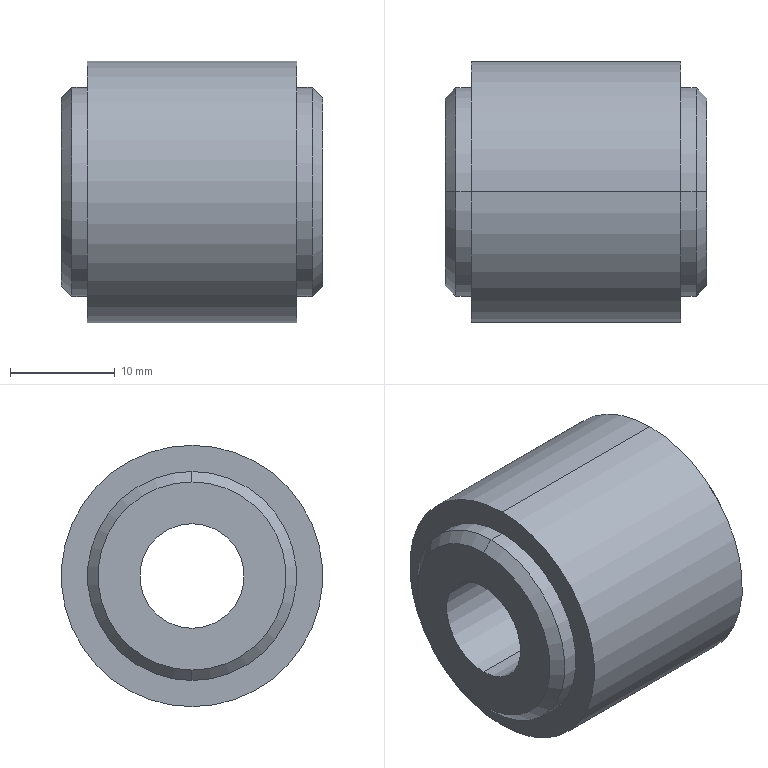Part | SolidWorks | features Chamfer 1, Extrusion 1, ICE 1 | 1 solid | 16 faces | box 25 x 25 x 25 mm | volume 9364 mm3 | cylinder 8 | cone 4 | plane 4 | commonest cylinder face diameters 20 x4 10 x2 25 x2
STEP:
#1=CARTESIAN_POINT('',(12.5,0.,-9.));
#2=VERTEX_POINT('',#1);
#3=CARTESIAN_POINT('',(12.5,0.,9.));
#4=VERTEX_POINT('',#3);
#5=CARTESIAN_POINT('',(12.5,0.,0.));
#6=DIRECTION('',(1.,0.,0.));
#7=DIRECTION('',(0.,0.,-1.));
#8=AXIS2_PLACEMENT_3D('',#5,#6,#7);
#9=CIRCLE('',#8,9.);
#10=EDGE_CURVE('',#2,#4,#9,.T.);
#11=ORIENTED_EDGE('',*,*,#10,.F.);
#12=CARTESIAN_POINT('',(11.5,0.,-10.));
#13=VERTEX_POINT('',#12);
#14=CARTESIAN_POINT('',(12.5,0.,-9.));
#15=DIRECTION('',(-0.7071,0.,-0.7071));
#16=VECTOR('',#15,1000.);
#17=LINE('',#14,#16);
#18=EDGE_CURVE('',#2,#13,#17,.T.);
#19=ORIENTED_EDGE('',*,*,#18,.T.);
#20=CARTESIAN_POINT('',(11.5,0.,10.));
#21=VERTEX_POINT('',#20);
#22=CARTESIAN_POINT('',(11.5,0.,0.));
#23=DIRECTION('',(-1.,0.,0.));
#24=DIRECTION('',(0.,0.,-1.));
#25=AXIS2_PLACEMENT_3D('',#22,#23,#24);
#26=CIRCLE('',#25,10.);
#27=EDGE_CURVE('',#21,#13,#26,.T.);
#28=ORIENTED_EDGE('',*,*,#27,.F.);
#29=CARTESIAN_POINT('',(12.5,0.,9.));
#30=DIRECTION('',(-0.7071,0.,0.7071));
#31=VECTOR('',#30,1000.);
#32=LINE('',#29,#31);
#33=EDGE_CURVE('',#4,#21,#32,.T.);
#34=ORIENTED_EDGE('',*,*,#33,.F.);
#35=EDGE_LOOP('',(#11,#19,#28,#34));
#36=FACE_OUTER_BOUND('',#35,.T.);
#37=CARTESIAN_POINT('',(12.5,0.,0.));
#38=DIRECTION('',(-1.,0.,0.));
#39=DIRECTION('',(0.,0.,1.));
#40=AXIS2_PLACEMENT_3D('',#37,#38,#39);
#41=CONICAL_SURFACE('',#40,9.,0.7854);
#42=ADVANCED_FACE('',(#36),#41,.T.);
#43=CARTESIAN_POINT('',(-12.5,0.,9.));
#44=VERTEX_POINT('',#43);
#45=CARTESIAN_POINT('',(-12.5,0.,-9.));
#46=VERTEX_POINT('',#45);
#47=CARTESIAN_POINT('',(-12.5,0.,0.));
#48=DIRECTION('',(-1.,0.,0.));
#49=DIRECTION('',(0.,0.,-1.));
#50=AXIS2_PLACEMENT_3D('',#47,#48,#49);
#51=CIRCLE('',#50,9.);
#52=EDGE_CURVE('',#44,#46,#51,.T.);
#53=ORIENTED_EDGE('',*,*,#52,.F.);
#54=CARTESIAN_POINT('',(-11.5,0.,10.));
#55=VERTEX_POINT('',#54);
#56=CARTESIAN_POINT('',(-11.5,0.,10.));
#57=DIRECTION('',(0.7071,0.,0.7071));
#58=VECTOR('',#57,1000.);
#59=LINE('',#56,#58);
#60=EDGE_CURVE('',#44,#55,#59,.T.);
#61=ORIENTED_EDGE('',*,*,#60,.T.);
#62=CARTESIAN_POINT('',(-11.5,0.,-10.));
#63=VERTEX_POINT('',#62);
#64=CARTESIAN_POINT('',(-11.5,0.,0.));
#65=DIRECTION('',(1.,0.,0.));
#66=DIRECTION('',(0.,0.,-1.));
#67=AXIS2_PLACEMENT_3D('',#64,#65,#66);
#68=CIRCLE('',#67,10.);
#69=EDGE_CURVE('',#63,#55,#68,.T.);
#70=ORIENTED_EDGE('',*,*,#69,.F.);
#71=CARTESIAN_POINT('',(-11.5,0.,-10.));
#72=DIRECTION('',(0.7071,0.,-0.7071));
#73=VECTOR('',#72,1000.);
#74=LINE('',#71,#73);
#75=EDGE_CURVE('',#46,#63,#74,.T.);
#76=ORIENTED_EDGE('',*,*,#75,.F.);
#77=EDGE_LOOP('',(#53,#61,#70,#76));
#78=FACE_OUTER_BOUND('',#77,.T.);
#79=CARTESIAN_POINT('',(-11.5,0.,0.));
#80=DIRECTION('',(1.,0.,0.));
#81=DIRECTION('',(0.,0.,-1.));
#82=AXIS2_PLACEMENT_3D('',#79,#80,#81);
#83=CONICAL_SURFACE('',#82,10.,0.7854);
#84=ADVANCED_FACE('',(#78),#83,.T.);
#85=CARTESIAN_POINT('',(10.,0.,-12.5));
#86=VERTEX_POINT('',#85);
#87=CARTESIAN_POINT('',(10.,0.,12.5));
#88=VERTEX_POINT('',#87);
#89=CARTESIAN_POINT('',(10.,0.,0.));
#90=DIRECTION('',(1.,0.,0.));
#91=DIRECTION('',(0.,0.,-1.));
#92=AXIS2_PLACEMENT_3D('',#89,#90,#91);
#93=CIRCLE('',#92,12.5);
#94=EDGE_CURVE('',#86,#88,#93,.T.);
#95=ORIENTED_EDGE('',*,*,#94,.F.);
#96=CARTESIAN_POINT('',(-10.,0.,-12.5));
#97=VERTEX_POINT('',#96);
#98=CARTESIAN_POINT('',(10.,0.,-12.5));
#99=DIRECTION('',(-1.,0.,0.));
#100=VECTOR('',#99,1000.);
#101=LINE('',#98,#100);
#102=EDGE_CURVE('',#86,#97,#101,.T.);
#103=ORIENTED_EDGE('',*,*,#102,.T.);
#104=CARTESIAN_POINT('',(-10.,0.,12.5));
#105=VERTEX_POINT('',#104);
#106=CARTESIAN_POINT('',(-10.,0.,0.));
#107=DIRECTION('',(1.,0.,0.));
#108=DIRECTION('',(0.,0.,-1.));
#109=AXIS2_PLACEMENT_3D('',#106,#107,#108);
#110=CIRCLE('',#109,12.5);
#111=EDGE_CURVE('',#97,#105,#110,.T.);
#112=ORIENTED_EDGE('',*,*,#111,.T.);
#113=CARTESIAN_POINT('',(10.,0.,12.5));
#114=DIRECTION('',(-1.,0.,0.));
#115=VECTOR('',#114,1000.);
#116=LINE('',#113,#115);
#117=EDGE_CURVE('',#88,#105,#116,.T.);
#118=ORIENTED_EDGE('',*,*,#117,.F.);
#119=EDGE_LOOP('',(#95,#103,#112,#118));
#120=FACE_OUTER_BOUND('',#119,.T.);
#121=CARTESIAN_POINT('',(10.,0.,0.));
#122=DIRECTION('',(-1.,0.,0.));
#123=DIRECTION('',(0.,0.,1.));
#124=AXIS2_PLACEMENT_3D('',#121,#122,#123);
#125=CYLINDRICAL_SURFACE('',#124,12.5);
#126=ADVANCED_FACE('',(#120),#125,.T.);
#127=CARTESIAN_POINT('',(12.5,0.,5.));
#128=VERTEX_POINT('',#127);
#129=CARTESIAN_POINT('',(12.5,0.,-5.));
#130=VERTEX_POINT('',#129);
#131=CARTESIAN_POINT('',(12.5,0.,0.));
#132=DIRECTION('',(1.,0.,0.));
#133=DIRECTION('',(0.,0.,-1.));
#134=AXIS2_PLACEMENT_3D('',#131,#132,#133);
#135=CIRCLE('',#134,5.);
#136=EDGE_CURVE('',#128,#130,#135,.T.);
#137=ORIENTED_EDGE('',*,*,#136,.T.);
#138=CARTESIAN_POINT('',(-12.5,0.,-5.));
#139=VERTEX_POINT('',#138);
#140=CARTESIAN_POINT('',(12.5,0.,-5.));
#141=DIRECTION('',(-1.,0.,0.));
#142=VECTOR('',#141,1000.);
#143=LINE('',#140,#142);
#144=EDGE_CURVE('',#130,#139,#143,.T.);
#145=ORIENTED_EDGE('',*,*,#144,.T.);
#146=CARTESIAN_POINT('',(-12.5,0.,5.));
#147=VERTEX_POINT('',#146);
#148=CARTESIAN_POINT('',(-12.5,0.,0.));
#149=DIRECTION('',(1.,0.,0.));
#150=DIRECTION('',(0.,0.,-1.));
#151=AXIS2_PLACEMENT_3D('',#148,#149,#150);
#152=CIRCLE('',#151,5.);
#153=EDGE_CURVE('',#147,#139,#152,.T.);
#154=ORIENTED_EDGE('',*,*,#153,.F.);
#155=CARTESIAN_POINT('',(12.5,0.,5.));
#156=DIRECTION('',(-1.,0.,0.));
#157=VECTOR('',#156,1000.);
#158=LINE('',#155,#157);
#159=EDGE_CURVE('',#128,#147,#158,.T.);
#160=ORIENTED_EDGE('',*,*,#159,.F.);
#161=EDGE_LOOP('',(#137,#145,#154,#160));
#162=FACE_OUTER_BOUND('',#161,.T.);
#163=CARTESIAN_POINT('',(12.5,0.,0.));
#164=DIRECTION('',(-1.,0.,0.));
#165=DIRECTION('',(0.,0.,1.));
#166=AXIS2_PLACEMENT_3D('',#163,#164,#165);
#167=CYLINDRICAL_SURFACE('',#166,5.);
#168=ADVANCED_FACE('',(#162),#167,.F.);
#169=ORIENTED_EDGE('',*,*,#27,.T.);
#170=CARTESIAN_POINT('',(10.,0.,-10.));
#171=VERTEX_POINT('',#170);
#172=CARTESIAN_POINT('',(12.5,0.,-10.));
#173=DIRECTION('',(-1.,0.,0.));
#174=VECTOR('',#173,1000.);
#175=LINE('',#172,#174);
#176=EDGE_CURVE('',#13,#171,#175,.T.);
#177=ORIENTED_EDGE('',*,*,#176,.T.);
#178=CARTESIAN_POINT('',(10.,0.,10.));
#179=VERTEX_POINT('',#178);
#180=CARTESIAN_POINT('',(10.,0.,0.));
#181=DIRECTION('',(1.,0.,0.));
#182=DIRECTION('',(0.,0.,-1.));
#183=AXIS2_PLACEMENT_3D('',#180,#181,#182);
#184=CIRCLE('',#183,10.);
#185=EDGE_CURVE('',#171,#179,#184,.T.);
#186=ORIENTED_EDGE('',*,*,#185,.T.);
#187=CARTESIAN_POINT('',(12.5,0.,10.));
#188=DIRECTION('',(-1.,0.,0.));
#189=VECTOR('',#188,1000.);
#190=LINE('',#187,#189);
#191=EDGE_CURVE('',#21,#179,#190,.T.);
#192=ORIENTED_EDGE('',*,*,#191,.F.);
#193=EDGE_LOOP('',(#169,#177,#186,#192));
#194=FACE_OUTER_BOUND('',#193,.T.);
#195=CARTESIAN_POINT('',(12.5,0.,0.));
#196=DIRECTION('',(-1.,0.,0.));
#197=DIRECTION('',(0.,0.,1.));
#198=AXIS2_PLACEMENT_3D('',#195,#196,#197);
#199=CYLINDRICAL_SURFACE('',#198,10.);
#200=ADVANCED_FACE('',(#194),#199,.T.);
#201=CARTESIAN_POINT('',(-10.,0.,-10.));
#202=VERTEX_POINT('',#201);
#203=CARTESIAN_POINT('',(-10.,0.,10.));
#204=VERTEX_POINT('',#203);
#205=CARTESIAN_POINT('',(-10.,0.,0.));
#206=DIRECTION('',(1.,0.,0.));
#207=DIRECTION('',(0.,0.,-1.));
#208=AXIS2_PLACEMENT_3D('',#205,#206,#207);
#209=CIRCLE('',#208,10.);
#210=EDGE_CURVE('',#202,#204,#209,.T.);
#211=ORIENTED_EDGE('',*,*,#210,.F.);
#212=CARTESIAN_POINT('',(12.5,0.,-10.));
#213=DIRECTION('',(-1.,0.,0.));
#214=VECTOR('',#213,1000.);
#215=LINE('',#212,#214);
#216=EDGE_CURVE('',#202,#63,#215,.T.);
#217=ORIENTED_EDGE('',*,*,#216,.T.);
#218=ORIENTED_EDGE('',*,*,#69,.T.);
#219=CARTESIAN_POINT('',(12.5,0.,10.));
#220=DIRECTION('',(-1.,0.,0.));
#221=VECTOR('',#220,1000.);
#222=LINE('',#219,#221);
#223=EDGE_CURVE('',#204,#55,#222,.T.);
#224=ORIENTED_EDGE('',*,*,#223,.F.);
#225=EDGE_LOOP('',(#211,#217,#218,#224));
#226=FACE_OUTER_BOUND('',#225,.T.);
#227=CARTESIAN_POINT('',(12.5,0.,0.));
#228=DIRECTION('',(-1.,0.,0.));
#229=DIRECTION('',(0.,0.,1.));
#230=AXIS2_PLACEMENT_3D('',#227,#228,#229);
#231=CYLINDRICAL_SURFACE('',#230,10.);
#232=ADVANCED_FACE('',(#226),#231,.T.);
#233=ORIENTED_EDGE('',*,*,#216,.F.);
#234=CARTESIAN_POINT('',(-10.,0.,0.));
#235=DIRECTION('',(1.,0.,0.));
#236=DIRECTION('',(0.,0.,-1.));
#237=AXIS2_PLACEMENT_3D('',#234,#235,#236);
#238=CIRCLE('',#237,10.);
#239=EDGE_CURVE('',#204,#202,#238,.T.);
#240=ORIENTED_EDGE('',*,*,#239,.F.);
#241=ORIENTED_EDGE('',*,*,#223,.T.);
#242=CARTESIAN_POINT('',(-11.5,0.,0.));
#243=DIRECTION('',(1.,0.,0.));
#244=DIRECTION('',(0.,0.,-1.));
#245=AXIS2_PLACEMENT_3D('',#242,#243,#244);
#246=CIRCLE('',#245,10.);
#247=EDGE_CURVE('',#55,#63,#246,.T.);
#248=ORIENTED_EDGE('',*,*,#247,.T.);
#249=EDGE_LOOP('',(#233,#240,#241,#248));
#250=FACE_OUTER_BOUND('',#249,.T.);
#251=CARTESIAN_POINT('',(12.5,0.,0.));
#252=DIRECTION('',(-1.,0.,0.));
#253=DIRECTION('',(0.,0.,1.));
#254=AXIS2_PLACEMENT_3D('',#251,#252,#253);
#255=CYLINDRICAL_SURFACE('',#254,10.);
#256=ADVANCED_FACE('',(#250),#255,.T.);
#257=CARTESIAN_POINT('',(12.5,0.,0.));
#258=DIRECTION('',(1.,0.,0.));
#259=DIRECTION('',(0.,0.,-1.));
#260=AXIS2_PLACEMENT_3D('',#257,#258,#259);
#261=CIRCLE('',#260,9.);
#262=EDGE_CURVE('',#4,#2,#261,.T.);
#263=ORIENTED_EDGE('',*,*,#262,.T.);
#264=ORIENTED_EDGE('',*,*,#10,.T.);
#265=EDGE_LOOP('',(#263,#264));
#266=FACE_OUTER_BOUND('',#265,.T.);
#267=ORIENTED_EDGE('',*,*,#136,.F.);
#268=CARTESIAN_POINT('',(12.5,0.,0.));
#269=DIRECTION('',(1.,0.,0.));
#270=DIRECTION('',(0.,0.,-1.));
#271=AXIS2_PLACEMENT_3D('',#268,#269,#270);
#272=CIRCLE('',#271,5.);
#273=EDGE_CURVE('',#130,#128,#272,.T.);
#274=ORIENTED_EDGE('',*,*,#273,.F.);
#275=EDGE_LOOP('',(#267,#274));
#276=FACE_BOUND('',#275,.T.);
#277=CARTESIAN_POINT('',(12.5,0.,0.));
#278=DIRECTION('',(1.,0.,0.));
#279=DIRECTION('',(0.,0.,-1.));
#280=AXIS2_PLACEMENT_3D('',#277,#278,#279);
#281=PLANE('',#280);
#282=ADVANCED_FACE('',(#266,#276),#281,.T.);
#283=CARTESIAN_POINT('',(-12.5,0.,0.));
#284=DIRECTION('',(-1.,0.,0.));
#285=DIRECTION('',(0.,0.,-1.));
#286=AXIS2_PLACEMENT_3D('',#283,#284,#285);
#287=CIRCLE('',#286,9.);
#288=EDGE_CURVE('',#46,#44,#287,.T.);
#289=ORIENTED_EDGE('',*,*,#288,.T.);
#290=ORIENTED_EDGE('',*,*,#52,.T.);
#291=EDGE_LOOP('',(#289,#290));
#292=FACE_OUTER_BOUND('',#291,.T.);
#293=ORIENTED_EDGE('',*,*,#153,.T.);
#294=CARTESIAN_POINT('',(-12.5,0.,0.));
#295=DIRECTION('',(1.,0.,0.));
#296=DIRECTION('',(0.,0.,-1.));
#297=AXIS2_PLACEMENT_3D('',#294,#295,#296);
#298=CIRCLE('',#297,5.);
#299=EDGE_CURVE('',#139,#147,#298,.T.);
#300=ORIENTED_EDGE('',*,*,#299,.T.);
#301=EDGE_LOOP('',(#293,#300));
#302=FACE_BOUND('',#301,.T.);
#303=CARTESIAN_POINT('',(-12.5,0.,0.));
#304=DIRECTION('',(1.,0.,0.));
#305=DIRECTION('',(0.,0.,-1.));
#306=AXIS2_PLACEMENT_3D('',#303,#304,#305);
#307=PLANE('',#306);
#308=ADVANCED_FACE('',(#292,#302),#307,.F.);
#309=ORIENTED_EDGE('',*,*,#176,.F.);
#310=CARTESIAN_POINT('',(11.5,0.,0.));
#311=DIRECTION('',(-1.,0.,0.));
#312=DIRECTION('',(0.,0.,-1.));
#313=AXIS2_PLACEMENT_3D('',#310,#311,#312);
#314=CIRCLE('',#313,10.);
#315=EDGE_CURVE('',#13,#21,#314,.T.);
#316=ORIENTED_EDGE('',*,*,#315,.T.);
#317=ORIENTED_EDGE('',*,*,#191,.T.);
#318=CARTESIAN_POINT('',(10.,0.,0.));
#319=DIRECTION('',(1.,0.,0.));
#320=DIRECTION('',(0.,0.,-1.));
#321=AXIS2_PLACEMENT_3D('',#318,#319,#320);
#322=CIRCLE('',#321,10.);
#323=EDGE_CURVE('',#179,#171,#322,.T.);
#324=ORIENTED_EDGE('',*,*,#323,.T.);
#325=EDGE_LOOP('',(#309,#316,#317,#324));
#326=FACE_OUTER_BOUND('',#325,.T.);
#327=CARTESIAN_POINT('',(12.5,0.,0.));
#328=DIRECTION('',(-1.,0.,0.));
#329=DIRECTION('',(0.,0.,1.));
#330=AXIS2_PLACEMENT_3D('',#327,#328,#329);
#331=CYLINDRICAL_SURFACE('',#330,10.);
#332=ADVANCED_FACE('',(#326),#331,.T.);
#333=ORIENTED_EDGE('',*,*,#144,.F.);
#334=ORIENTED_EDGE('',*,*,#273,.T.);
#335=ORIENTED_EDGE('',*,*,#159,.T.);
#336=ORIENTED_EDGE('',*,*,#299,.F.);
#337=EDGE_LOOP('',(#333,#334,#335,#336));
#338=FACE_OUTER_BOUND('',#337,.T.);
#339=CARTESIAN_POINT('',(12.5,0.,0.));
#340=DIRECTION('',(-1.,0.,0.));
#341=DIRECTION('',(0.,0.,1.));
#342=AXIS2_PLACEMENT_3D('',#339,#340,#341);
#343=CYLINDRICAL_SURFACE('',#342,5.);
#344=ADVANCED_FACE('',(#338),#343,.F.);
#345=CARTESIAN_POINT('',(10.,0.,0.));
#346=DIRECTION('',(1.,0.,0.));
#347=DIRECTION('',(0.,0.,-1.));
#348=AXIS2_PLACEMENT_3D('',#345,#346,#347);
#349=CIRCLE('',#348,12.5);
#350=EDGE_CURVE('',#88,#86,#349,.T.);
#351=ORIENTED_EDGE('',*,*,#350,.T.);
#352=ORIENTED_EDGE('',*,*,#94,.T.);
#353=EDGE_LOOP('',(#351,#352));
#354=FACE_OUTER_BOUND('',#353,.T.);
#355=ORIENTED_EDGE('',*,*,#323,.F.);
#356=ORIENTED_EDGE('',*,*,#185,.F.);
#357=EDGE_LOOP('',(#355,#356));
#358=FACE_BOUND('',#357,.T.);
#359=CARTESIAN_POINT('',(10.,0.,0.));
#360=DIRECTION('',(1.,0.,0.));
#361=DIRECTION('',(0.,0.,-1.));
#362=AXIS2_PLACEMENT_3D('',#359,#360,#361);
#363=PLANE('',#362);
#364=ADVANCED_FACE('',(#354,#358),#363,.T.);
#365=CARTESIAN_POINT('',(-10.,0.,0.));
#366=DIRECTION('',(1.,0.,0.));
#367=DIRECTION('',(0.,0.,-1.));
#368=AXIS2_PLACEMENT_3D('',#365,#366,#367);
#369=CIRCLE('',#368,12.5);
#370=EDGE_CURVE('',#105,#97,#369,.T.);
#371=ORIENTED_EDGE('',*,*,#370,.F.);
#372=ORIENTED_EDGE('',*,*,#111,.F.);
#373=EDGE_LOOP('',(#371,#372));
#374=FACE_OUTER_BOUND('',#373,.T.);
#375=ORIENTED_EDGE('',*,*,#239,.T.);
#376=ORIENTED_EDGE('',*,*,#210,.T.);
#377=EDGE_LOOP('',(#375,#376));
#378=FACE_BOUND('',#377,.T.);
#379=CARTESIAN_POINT('',(-10.,0.,0.));
#380=DIRECTION('',(1.,0.,0.));
#381=DIRECTION('',(0.,0.,-1.));
#382=AXIS2_PLACEMENT_3D('',#379,#380,#381);
#383=PLANE('',#382);
#384=ADVANCED_FACE('',(#374,#378),#383,.F.);
#385=ORIENTED_EDGE('',*,*,#102,.F.);
#386=ORIENTED_EDGE('',*,*,#350,.F.);
#387=ORIENTED_EDGE('',*,*,#117,.T.);
#388=ORIENTED_EDGE('',*,*,#370,.T.);
#389=EDGE_LOOP('',(#385,#386,#387,#388));
#390=FACE_OUTER_BOUND('',#389,.T.);
#391=CARTESIAN_POINT('',(10.,0.,0.));
#392=DIRECTION('',(-1.,0.,0.));
#393=DIRECTION('',(0.,0.,1.));
#394=AXIS2_PLACEMENT_3D('',#391,#392,#393);
#395=CYLINDRICAL_SURFACE('',#394,12.5);
#396=ADVANCED_FACE('',(#390),#395,.T.);
#397=ORIENTED_EDGE('',*,*,#60,.F.);
#398=ORIENTED_EDGE('',*,*,#288,.F.);
#399=ORIENTED_EDGE('',*,*,#75,.T.);
#400=ORIENTED_EDGE('',*,*,#247,.F.);
#401=EDGE_LOOP('',(#397,#398,#399,#400));
#402=FACE_OUTER_BOUND('',#401,.T.);
#403=CARTESIAN_POINT('',(-11.5,0.,0.));
#404=DIRECTION('',(1.,0.,0.));
#405=DIRECTION('',(0.,0.,-1.));
#406=AXIS2_PLACEMENT_3D('',#403,#404,#405);
#407=CONICAL_SURFACE('',#406,10.,0.7854);
#408=ADVANCED_FACE('',(#402),#407,.T.);
#409=ORIENTED_EDGE('',*,*,#18,.F.);
#410=ORIENTED_EDGE('',*,*,#262,.F.);
#411=ORIENTED_EDGE('',*,*,#33,.T.);
#412=ORIENTED_EDGE('',*,*,#315,.F.);
#413=EDGE_LOOP('',(#409,#410,#411,#412));
#414=FACE_OUTER_BOUND('',#413,.T.);
#415=CARTESIAN_POINT('',(12.5,0.,0.));
#416=DIRECTION('',(-1.,0.,0.));
#417=DIRECTION('',(0.,0.,1.));
#418=AXIS2_PLACEMENT_3D('',#415,#416,#417);
#419=CONICAL_SURFACE('',#418,9.,0.7854);
#420=ADVANCED_FACE('',(#414),#419,.T.);
#421=CLOSED_SHELL('',(#42,#84,#126,#168,#200,#232,#256,#282,#308,#332,#344,#364,#384,#396,#408,#420));
#422=MANIFOLD_SOLID_BREP('',#421);
#423=CARTESIAN_POINT('',(0.,0.,0.));
#424=DIRECTION('',(0.,0.,1.));
#425=DIRECTION('',(1.,0.,0.));
#426=AXIS2_PLACEMENT_3D('',#423,#424,#425);
#427=(LENGTH_UNIT()NAMED_UNIT(*)SI_UNIT(.MILLI.,.METRE.));
#428=UNCERTAINTY_MEASURE_WITH_UNIT(LENGTH_MEASURE(0.00001),#427,'','');
#429=(NAMED_UNIT(*)PLANE_ANGLE_UNIT()SI_UNIT($,.RADIAN.));
#430=(NAMED_UNIT(*)SI_UNIT($,.STERADIAN.)SOLID_ANGLE_UNIT());
#431=(GEOMETRIC_REPRESENTATION_CONTEXT(3)GLOBAL_UNCERTAINTY_ASSIGNED_CONTEXT((#428))GLOBAL_UNIT_ASSIGNED_CONTEXT((#427,#429,#430))REPRESENTATION_CONTEXT('',''));
#432=ADVANCED_BREP_SHAPE_REPRESENTATION('',(#422,#426),#431);